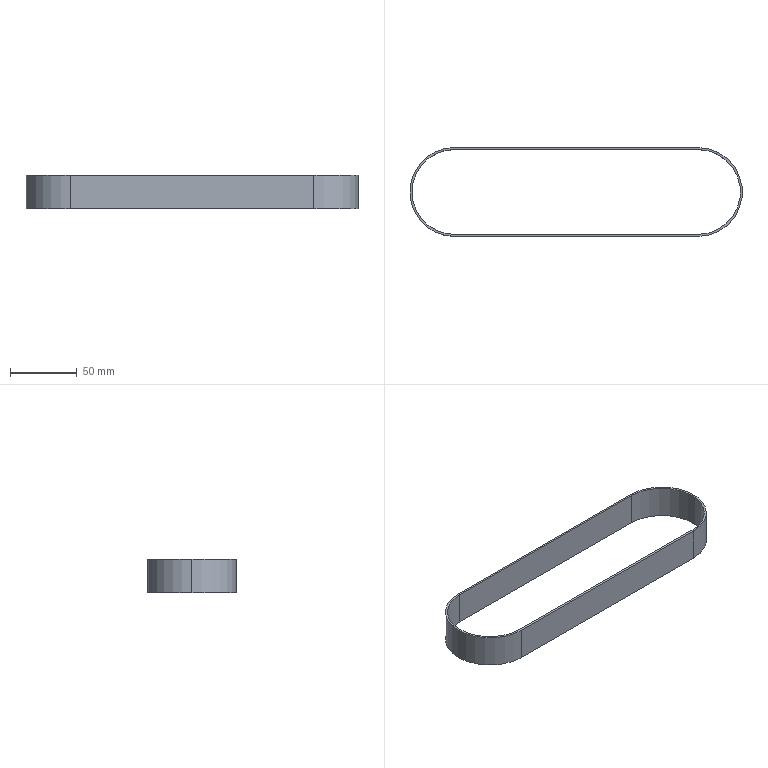Part | STEP file | Timing belt S5M-width 25-length 565 (steel wire core) | 1 solid | 12 faces | box 249.2 x 66.7 x 25 mm | volume 21369 mm3 | cylinder 6 | plane 6 | commonest cylinder face diameters 63.7 x3 66.7 x3
STEP:
#1=CARTESIAN_POINT('',(0.,0.,0.));
#2=DIRECTION('',(0.,0.,1.));
#3=DIRECTION('',(1.,0.,0.));
#4=AXIS2_PLACEMENT_3D('',#1,#2,#3);
#5=CARTESIAN_POINT('',(-91.25,31.85,12.5));
#6=VERTEX_POINT('',#5);
#7=CARTESIAN_POINT('',(-91.25,31.85,-12.5));
#8=VERTEX_POINT('',#7);
#9=CARTESIAN_POINT('',(-91.25,31.85,12.5));
#10=DIRECTION('',(0.,0.,-1.));
#11=VECTOR('',#10,1.);
#12=LINE('',#9,#11);
#13=CARTESIAN_POINT('',(-91.25,0.,12.5));
#14=DIRECTION('',(0.,0.,-1.));
#15=DIRECTION('',(-1.,0.,0.));
#16=AXIS2_PLACEMENT_3D('',#13,#14,#15);
#17=CYLINDRICAL_SURFACE('',#16,31.85);
#18=CARTESIAN_POINT('',(1.571,0.));
#19=DIRECTION('',(0.,1.));
#20=VECTOR('',#19,1.);
#21=LINE('',#18,#20);
#22=(GEOMETRIC_REPRESENTATION_CONTEXT(2)PARAMETRIC_REPRESENTATION_CONTEXT()REPRESENTATION_CONTEXT('',''));
#23=DEFINITIONAL_REPRESENTATION('',(#21),#22);
#24=PCURVE('',#17,#23);
#25=CARTESIAN_POINT('',(-91.25,31.85,12.5));
#26=DIRECTION('',(0.,-1.,0.));
#27=DIRECTION('',(0.,0.,-1.));
#28=AXIS2_PLACEMENT_3D('',#25,#26,#27);
#29=PLANE('',#28);
#30=CARTESIAN_POINT('',(0.,0.));
#31=DIRECTION('',(1.,0.));
#32=VECTOR('',#31,1.);
#33=LINE('',#30,#32);
#34=(GEOMETRIC_REPRESENTATION_CONTEXT(2)PARAMETRIC_REPRESENTATION_CONTEXT()REPRESENTATION_CONTEXT('',''));
#35=DEFINITIONAL_REPRESENTATION('',(#33),#34);
#36=PCURVE('',#29,#35);
#37=SURFACE_CURVE('',#12,(#24,#36),.PCURVE_S1.);
#38=EDGE_CURVE('',#6,#8,#37,.T.);
#39=ORIENTED_EDGE('',*,*,#38,.T.);
#40=CARTESIAN_POINT('',(-123.1,0.,-12.5));
#41=VERTEX_POINT('',#40);
#42=CARTESIAN_POINT('',(-91.25,0.,-12.5));
#43=DIRECTION('',(0.,0.,1.));
#44=DIRECTION('',(1.,0.,0.));
#45=AXIS2_PLACEMENT_3D('',#42,#43,#44);
#46=CIRCLE('',#45,31.85);
#47=CARTESIAN_POINT('',(3.142,25.));
#48=DIRECTION('',(-1.,0.));
#49=VECTOR('',#48,1.);
#50=LINE('',#47,#49);
#51=(GEOMETRIC_REPRESENTATION_CONTEXT(2)PARAMETRIC_REPRESENTATION_CONTEXT()REPRESENTATION_CONTEXT('',''));
#52=DEFINITIONAL_REPRESENTATION('',(#50),#51);
#53=PCURVE('',#17,#52);
#54=CARTESIAN_POINT('',(-91.25,0.,-12.5));
#55=DIRECTION('',(0.,0.,1.));
#56=DIRECTION('',(1.,0.,0.));
#57=AXIS2_PLACEMENT_3D('',#54,#55,#56);
#58=PLANE('',#57);
#59=CARTESIAN_POINT('',(0.,0.));
#60=DIRECTION('',(1.,0.));
#61=AXIS2_PLACEMENT_2D('',#59,#60);
#62=CIRCLE('',#61,31.85);
#63=(GEOMETRIC_REPRESENTATION_CONTEXT(2)PARAMETRIC_REPRESENTATION_CONTEXT()REPRESENTATION_CONTEXT('',''));
#64=DEFINITIONAL_REPRESENTATION('',(#62),#63);
#65=PCURVE('',#58,#64);
#66=SURFACE_CURVE('',#46,(#53,#65),.PCURVE_S1.);
#67=EDGE_CURVE('',#8,#41,#66,.T.);
#68=ORIENTED_EDGE('',*,*,#67,.T.);
#69=CARTESIAN_POINT('',(-123.1,0.,12.5));
#70=VERTEX_POINT('',#69);
#71=CARTESIAN_POINT('',(-123.1,0.,12.5));
#72=DIRECTION('',(0.,0.,-1.));
#73=VECTOR('',#72,1.);
#74=LINE('',#71,#73);
#75=CARTESIAN_POINT('',(0.,0.));
#76=DIRECTION('',(0.,1.));
#77=VECTOR('',#76,1.);
#78=LINE('',#75,#77);
#79=(GEOMETRIC_REPRESENTATION_CONTEXT(2)PARAMETRIC_REPRESENTATION_CONTEXT()REPRESENTATION_CONTEXT('',''));
#80=DEFINITIONAL_REPRESENTATION('',(#78),#79);
#81=PCURVE('',#17,#80);
#82=CARTESIAN_POINT('',(-91.25,0.,12.5));
#83=DIRECTION('',(0.,0.,-1.));
#84=DIRECTION('',(-1.,0.,0.));
#85=AXIS2_PLACEMENT_3D('',#82,#83,#84);
#86=CYLINDRICAL_SURFACE('',#85,31.85);
#87=CARTESIAN_POINT('',(6.283,0.));
#88=DIRECTION('',(0.,1.));
#89=VECTOR('',#88,1.);
#90=LINE('',#87,#89);
#91=(GEOMETRIC_REPRESENTATION_CONTEXT(2)PARAMETRIC_REPRESENTATION_CONTEXT()REPRESENTATION_CONTEXT('',''));
#92=DEFINITIONAL_REPRESENTATION('',(#90),#91);
#93=PCURVE('',#86,#92);
#94=SURFACE_CURVE('',#74,(#81,#93),.PCURVE_S1.);
#95=EDGE_CURVE('',#70,#41,#94,.T.);
#96=ORIENTED_EDGE('',*,*,#95,.F.);
#97=CARTESIAN_POINT('',(-91.25,0.,12.5));
#98=DIRECTION('',(0.,0.,1.));
#99=DIRECTION('',(1.,0.,0.));
#100=AXIS2_PLACEMENT_3D('',#97,#98,#99);
#101=CIRCLE('',#100,31.85);
#102=CARTESIAN_POINT('',(3.142,0.));
#103=DIRECTION('',(-1.,0.));
#104=VECTOR('',#103,1.);
#105=LINE('',#102,#104);
#106=(GEOMETRIC_REPRESENTATION_CONTEXT(2)PARAMETRIC_REPRESENTATION_CONTEXT()REPRESENTATION_CONTEXT('',''));
#107=DEFINITIONAL_REPRESENTATION('',(#105),#106);
#108=PCURVE('',#17,#107);
#109=CARTESIAN_POINT('',(-91.25,0.,12.5));
#110=DIRECTION('',(0.,0.,1.));
#111=DIRECTION('',(1.,0.,0.));
#112=AXIS2_PLACEMENT_3D('',#109,#110,#111);
#113=PLANE('',#112);
#114=CARTESIAN_POINT('',(0.,0.));
#115=DIRECTION('',(1.,0.));
#116=AXIS2_PLACEMENT_2D('',#114,#115);
#117=CIRCLE('',#116,31.85);
#118=(GEOMETRIC_REPRESENTATION_CONTEXT(2)PARAMETRIC_REPRESENTATION_CONTEXT()REPRESENTATION_CONTEXT('',''));
#119=DEFINITIONAL_REPRESENTATION('',(#117),#118);
#120=PCURVE('',#113,#119);
#121=SURFACE_CURVE('',#101,(#108,#120),.PCURVE_S1.);
#122=EDGE_CURVE('',#6,#70,#121,.T.);
#123=ORIENTED_EDGE('',*,*,#122,.F.);
#124=EDGE_LOOP('',(#39,#68,#96,#123));
#125=FACE_BOUND('',#124,.F.);
#126=ADVANCED_FACE('',(#125),#17,.F.);
#127=CARTESIAN_POINT('',(-124.6,0.,12.5));
#128=VERTEX_POINT('',#127);
#129=CARTESIAN_POINT('',(-91.25,-33.35,12.5));
#130=VERTEX_POINT('',#129);
#131=CARTESIAN_POINT('',(-91.25,0.,12.5));
#132=DIRECTION('',(0.,0.,1.));
#133=DIRECTION('',(1.,0.,0.));
#134=AXIS2_PLACEMENT_3D('',#131,#132,#133);
#135=CIRCLE('',#134,33.35);
#136=CARTESIAN_POINT('',(-91.25,0.,12.5));
#137=DIRECTION('',(0.,0.,-1.));
#138=DIRECTION('',(-1.,0.,0.));
#139=AXIS2_PLACEMENT_3D('',#136,#137,#138);
#140=CYLINDRICAL_SURFACE('',#139,33.35);
#141=CARTESIAN_POINT('',(9.425,0.));
#142=DIRECTION('',(-1.,0.));
#143=VECTOR('',#142,1.);
#144=LINE('',#141,#143);
#145=(GEOMETRIC_REPRESENTATION_CONTEXT(2)PARAMETRIC_REPRESENTATION_CONTEXT()REPRESENTATION_CONTEXT('',''));
#146=DEFINITIONAL_REPRESENTATION('',(#144),#145);
#147=PCURVE('',#140,#146);
#148=CARTESIAN_POINT('',(0.,0.));
#149=DIRECTION('',(1.,0.));
#150=AXIS2_PLACEMENT_2D('',#148,#149);
#151=CIRCLE('',#150,33.35);
#152=(GEOMETRIC_REPRESENTATION_CONTEXT(2)PARAMETRIC_REPRESENTATION_CONTEXT()REPRESENTATION_CONTEXT('',''));
#153=DEFINITIONAL_REPRESENTATION('',(#151),#152);
#154=PCURVE('',#113,#153);
#155=SURFACE_CURVE('',#135,(#147,#154),.PCURVE_S1.);
#156=EDGE_CURVE('',#128,#130,#155,.T.);
#157=ORIENTED_EDGE('',*,*,#156,.F.);
#158=CARTESIAN_POINT('',(-124.6,0.,-12.5));
#159=VERTEX_POINT('',#158);
#160=CARTESIAN_POINT('',(-124.6,0.,12.5));
#161=DIRECTION('',(0.,0.,-1.));
#162=VECTOR('',#161,1.);
#163=LINE('',#160,#162);
#164=CARTESIAN_POINT('',(6.283,0.));
#165=DIRECTION('',(0.,1.));
#166=VECTOR('',#165,1.);
#167=LINE('',#164,#166);
#168=(GEOMETRIC_REPRESENTATION_CONTEXT(2)PARAMETRIC_REPRESENTATION_CONTEXT()REPRESENTATION_CONTEXT('',''));
#169=DEFINITIONAL_REPRESENTATION('',(#167),#168);
#170=PCURVE('',#140,#169);
#171=CARTESIAN_POINT('',(-91.25,0.,12.5));
#172=DIRECTION('',(0.,0.,-1.));
#173=DIRECTION('',(-1.,0.,0.));
#174=AXIS2_PLACEMENT_3D('',#171,#172,#173);
#175=CYLINDRICAL_SURFACE('',#174,33.35);
#176=CARTESIAN_POINT('',(0.,0.));
#177=DIRECTION('',(0.,1.));
#178=VECTOR('',#177,1.);
#179=LINE('',#176,#178);
#180=(GEOMETRIC_REPRESENTATION_CONTEXT(2)PARAMETRIC_REPRESENTATION_CONTEXT()REPRESENTATION_CONTEXT('',''));
#181=DEFINITIONAL_REPRESENTATION('',(#179),#180);
#182=PCURVE('',#175,#181);
#183=SURFACE_CURVE('',#163,(#170,#182),.PCURVE_S1.);
#184=EDGE_CURVE('',#128,#159,#183,.T.);
#185=ORIENTED_EDGE('',*,*,#184,.T.);
#186=CARTESIAN_POINT('',(-91.25,-33.35,-12.5));
#187=VERTEX_POINT('',#186);
#188=CARTESIAN_POINT('',(-91.25,0.,-12.5));
#189=DIRECTION('',(0.,0.,1.));
#190=DIRECTION('',(1.,0.,0.));
#191=AXIS2_PLACEMENT_3D('',#188,#189,#190);
#192=CIRCLE('',#191,33.35);
#193=CARTESIAN_POINT('',(9.425,25.));
#194=DIRECTION('',(-1.,0.));
#195=VECTOR('',#194,1.);
#196=LINE('',#193,#195);
#197=(GEOMETRIC_REPRESENTATION_CONTEXT(2)PARAMETRIC_REPRESENTATION_CONTEXT()REPRESENTATION_CONTEXT('',''));
#198=DEFINITIONAL_REPRESENTATION('',(#196),#197);
#199=PCURVE('',#140,#198);
#200=CARTESIAN_POINT('',(0.,0.));
#201=DIRECTION('',(1.,0.));
#202=AXIS2_PLACEMENT_2D('',#200,#201);
#203=CIRCLE('',#202,33.35);
#204=(GEOMETRIC_REPRESENTATION_CONTEXT(2)PARAMETRIC_REPRESENTATION_CONTEXT()REPRESENTATION_CONTEXT('',''));
#205=DEFINITIONAL_REPRESENTATION('',(#203),#204);
#206=PCURVE('',#58,#205);
#207=SURFACE_CURVE('',#192,(#199,#206),.PCURVE_S1.);
#208=EDGE_CURVE('',#159,#187,#207,.T.);
#209=ORIENTED_EDGE('',*,*,#208,.T.);
#210=CARTESIAN_POINT('',(-91.25,-33.35,12.5));
#211=DIRECTION('',(0.,0.,-1.));
#212=VECTOR('',#211,1.);
#213=LINE('',#210,#212);
#214=CARTESIAN_POINT('',(4.712,0.));
#215=DIRECTION('',(0.,1.));
#216=VECTOR('',#215,1.);
#217=LINE('',#214,#216);
#218=(GEOMETRIC_REPRESENTATION_CONTEXT(2)PARAMETRIC_REPRESENTATION_CONTEXT()REPRESENTATION_CONTEXT('',''));
#219=DEFINITIONAL_REPRESENTATION('',(#217),#218);
#220=PCURVE('',#140,#219);
#221=CARTESIAN_POINT('',(-91.25,-33.35,12.5));
#222=DIRECTION('',(0.,1.,0.));
#223=DIRECTION('',(0.,0.,1.));
#224=AXIS2_PLACEMENT_3D('',#221,#222,#223);
#225=PLANE('',#224);
#226=CARTESIAN_POINT('',(0.,0.));
#227=DIRECTION('',(-1.,0.));
#228=VECTOR('',#227,1.);
#229=LINE('',#226,#228);
#230=(GEOMETRIC_REPRESENTATION_CONTEXT(2)PARAMETRIC_REPRESENTATION_CONTEXT()REPRESENTATION_CONTEXT('',''));
#231=DEFINITIONAL_REPRESENTATION('',(#229),#230);
#232=PCURVE('',#225,#231);
#233=SURFACE_CURVE('',#213,(#220,#232),.PCURVE_S1.);
#234=EDGE_CURVE('',#130,#187,#233,.T.);
#235=ORIENTED_EDGE('',*,*,#234,.F.);
#236=EDGE_LOOP('',(#157,#185,#209,#235));
#237=FACE_BOUND('',#236,.T.);
#238=ADVANCED_FACE('',(#237),#140,.T.);
#239=CARTESIAN_POINT('',(-91.25,33.35,12.5));
#240=VERTEX_POINT('',#239);
#241=CARTESIAN_POINT('',(-91.25,0.,12.5));
#242=DIRECTION('',(0.,0.,1.));
#243=DIRECTION('',(1.,0.,0.));
#244=AXIS2_PLACEMENT_3D('',#241,#242,#243);
#245=CIRCLE('',#244,33.35);
#246=CARTESIAN_POINT('',(0.,0.));
#247=DIRECTION('',(1.,0.));
#248=AXIS2_PLACEMENT_2D('',#246,#247);
#249=CIRCLE('',#248,33.35);
#250=(GEOMETRIC_REPRESENTATION_CONTEXT(2)PARAMETRIC_REPRESENTATION_CONTEXT()REPRESENTATION_CONTEXT('',''));
#251=DEFINITIONAL_REPRESENTATION('',(#249),#250);
#252=PCURVE('',#113,#251);
#253=CARTESIAN_POINT('',(3.142,0.));
#254=DIRECTION('',(-1.,0.));
#255=VECTOR('',#254,1.);
#256=LINE('',#253,#255);
#257=(GEOMETRIC_REPRESENTATION_CONTEXT(2)PARAMETRIC_REPRESENTATION_CONTEXT()REPRESENTATION_CONTEXT('',''));
#258=DEFINITIONAL_REPRESENTATION('',(#256),#257);
#259=PCURVE('',#175,#258);
#260=SURFACE_CURVE('',#245,(#252,#259),.PCURVE_S1.);
#261=EDGE_CURVE('',#240,#128,#260,.T.);
#262=ORIENTED_EDGE('',*,*,#261,.T.);
#263=ORIENTED_EDGE('',*,*,#156,.T.);
#264=CARTESIAN_POINT('',(91.25,-33.35,12.5));
#265=VERTEX_POINT('',#264);
#266=CARTESIAN_POINT('',(-91.25,-33.35,12.5));
#267=DIRECTION('',(1.,0.,0.));
#268=VECTOR('',#267,1.);
#269=LINE('',#266,#268);
#270=CARTESIAN_POINT('',(0.,-33.35));
#271=DIRECTION('',(1.,0.));
#272=VECTOR('',#271,1.);
#273=LINE('',#270,#272);
#274=(GEOMETRIC_REPRESENTATION_CONTEXT(2)PARAMETRIC_REPRESENTATION_CONTEXT()REPRESENTATION_CONTEXT('',''));
#275=DEFINITIONAL_REPRESENTATION('',(#273),#274);
#276=PCURVE('',#113,#275);
#277=CARTESIAN_POINT('',(0.,0.));
#278=DIRECTION('',(0.,1.));
#279=VECTOR('',#278,1.);
#280=LINE('',#277,#279);
#281=(GEOMETRIC_REPRESENTATION_CONTEXT(2)PARAMETRIC_REPRESENTATION_CONTEXT()REPRESENTATION_CONTEXT('',''));
#282=DEFINITIONAL_REPRESENTATION('',(#280),#281);
#283=PCURVE('',#225,#282);
#284=SURFACE_CURVE('',#269,(#276,#283),.PCURVE_S1.);
#285=EDGE_CURVE('',#130,#265,#284,.T.);
#286=ORIENTED_EDGE('',*,*,#285,.T.);
#287=CARTESIAN_POINT('',(91.25,33.35,12.5));
#288=VERTEX_POINT('',#287);
#289=CARTESIAN_POINT('',(91.25,0.,12.5));
#290=DIRECTION('',(0.,0.,1.));
#291=DIRECTION('',(1.,0.,0.));
#292=AXIS2_PLACEMENT_3D('',#289,#290,#291);
#293=CIRCLE('',#292,33.35);
#294=CARTESIAN_POINT('',(182.5,0.));
#295=DIRECTION('',(1.,0.));
#296=AXIS2_PLACEMENT_2D('',#294,#295);
#297=CIRCLE('',#296,33.35);
#298=(GEOMETRIC_REPRESENTATION_CONTEXT(2)PARAMETRIC_REPRESENTATION_CONTEXT()REPRESENTATION_CONTEXT('',''));
#299=DEFINITIONAL_REPRESENTATION('',(#297),#298);
#300=PCURVE('',#113,#299);
#301=CARTESIAN_POINT('',(91.25,0.,12.5));
#302=DIRECTION('',(0.,0.,-1.));
#303=DIRECTION('',(-1.,0.,0.));
#304=AXIS2_PLACEMENT_3D('',#301,#302,#303);
#305=CYLINDRICAL_SURFACE('',#304,33.35);
#306=CARTESIAN_POINT('',(9.425,0.));
#307=DIRECTION('',(-1.,0.));
#308=VECTOR('',#307,1.);
#309=LINE('',#306,#308);
#310=(GEOMETRIC_REPRESENTATION_CONTEXT(2)PARAMETRIC_REPRESENTATION_CONTEXT()REPRESENTATION_CONTEXT('',''));
#311=DEFINITIONAL_REPRESENTATION('',(#309),#310);
#312=PCURVE('',#305,#311);
#313=SURFACE_CURVE('',#293,(#300,#312),.PCURVE_S1.);
#314=EDGE_CURVE('',#265,#288,#313,.T.);
#315=ORIENTED_EDGE('',*,*,#314,.T.);
#316=CARTESIAN_POINT('',(-91.25,33.35,12.5));
#317=DIRECTION('',(-1.,0.,0.));
#318=VECTOR('',#317,1.);
#319=LINE('',#316,#318);
#320=CARTESIAN_POINT('',(0.,33.35));
#321=DIRECTION('',(-1.,0.));
#322=VECTOR('',#321,1.);
#323=LINE('',#320,#322);
#324=(GEOMETRIC_REPRESENTATION_CONTEXT(2)PARAMETRIC_REPRESENTATION_CONTEXT()REPRESENTATION_CONTEXT('',''));
#325=DEFINITIONAL_REPRESENTATION('',(#323),#324);
#326=PCURVE('',#113,#325);
#327=CARTESIAN_POINT('',(-91.25,33.35,12.5));
#328=DIRECTION('',(0.,-1.,0.));
#329=DIRECTION('',(0.,0.,-1.));
#330=AXIS2_PLACEMENT_3D('',#327,#328,#329);
#331=PLANE('',#330);
#332=CARTESIAN_POINT('',(0.,0.));
#333=DIRECTION('',(0.,-1.));
#334=VECTOR('',#333,1.);
#335=LINE('',#332,#334);
#336=(GEOMETRIC_REPRESENTATION_CONTEXT(2)PARAMETRIC_REPRESENTATION_CONTEXT()REPRESENTATION_CONTEXT('',''));
#337=DEFINITIONAL_REPRESENTATION('',(#335),#336);
#338=PCURVE('',#331,#337);
#339=SURFACE_CURVE('',#319,(#326,#338),.PCURVE_S1.);
#340=EDGE_CURVE('',#288,#240,#339,.T.);
#341=ORIENTED_EDGE('',*,*,#340,.T.);
#342=EDGE_LOOP('',(#262,#263,#286,#315,#341));
#343=FACE_BOUND('',#342,.T.);
#344=CARTESIAN_POINT('',(-91.25,-31.85,12.5));
#345=VERTEX_POINT('',#344);
#346=CARTESIAN_POINT('',(91.25,-31.85,12.5));
#347=VERTEX_POINT('',#346);
#348=CARTESIAN_POINT('',(-91.25,-31.85,12.5));
#349=DIRECTION('',(1.,0.,0.));
#350=VECTOR('',#349,1.);
#351=LINE('',#348,#350);
#352=CARTESIAN_POINT('',(0.,-31.85));
#353=DIRECTION('',(1.,0.));
#354=VECTOR('',#353,1.);
#355=LINE('',#352,#354);
#356=(GEOMETRIC_REPRESENTATION_CONTEXT(2)PARAMETRIC_REPRESENTATION_CONTEXT()REPRESENTATION_CONTEXT('',''));
#357=DEFINITIONAL_REPRESENTATION('',(#355),#356);
#358=PCURVE('',#113,#357);
#359=CARTESIAN_POINT('',(-91.25,-31.85,12.5));
#360=DIRECTION('',(0.,1.,0.));
#361=DIRECTION('',(0.,0.,1.));
#362=AXIS2_PLACEMENT_3D('',#359,#360,#361);
#363=PLANE('',#362);
#364=CARTESIAN_POINT('',(0.,0.));
#365=DIRECTION('',(0.,1.));
#366=VECTOR('',#365,1.);
#367=LINE('',#364,#366);
#368=(GEOMETRIC_REPRESENTATION_CONTEXT(2)PARAMETRIC_REPRESENTATION_CONTEXT()REPRESENTATION_CONTEXT('',''));
#369=DEFINITIONAL_REPRESENTATION('',(#367),#368);
#370=PCURVE('',#363,#369);
#371=SURFACE_CURVE('',#351,(#358,#370),.PCURVE_S1.);
#372=EDGE_CURVE('',#345,#347,#371,.T.);
#373=ORIENTED_EDGE('',*,*,#372,.F.);
#374=CARTESIAN_POINT('',(-91.25,0.,12.5));
#375=DIRECTION('',(0.,0.,1.));
#376=DIRECTION('',(1.,0.,0.));
#377=AXIS2_PLACEMENT_3D('',#374,#375,#376);
#378=CIRCLE('',#377,31.85);
#379=CARTESIAN_POINT('',(0.,0.));
#380=DIRECTION('',(1.,0.));
#381=AXIS2_PLACEMENT_2D('',#379,#380);
#382=CIRCLE('',#381,31.85);
#383=(GEOMETRIC_REPRESENTATION_CONTEXT(2)PARAMETRIC_REPRESENTATION_CONTEXT()REPRESENTATION_CONTEXT('',''));
#384=DEFINITIONAL_REPRESENTATION('',(#382),#383);
#385=PCURVE('',#113,#384);
#386=CARTESIAN_POINT('',(9.425,0.));
#387=DIRECTION('',(-1.,0.));
#388=VECTOR('',#387,1.);
#389=LINE('',#386,#388);
#390=(GEOMETRIC_REPRESENTATION_CONTEXT(2)PARAMETRIC_REPRESENTATION_CONTEXT()REPRESENTATION_CONTEXT('',''));
#391=DEFINITIONAL_REPRESENTATION('',(#389),#390);
#392=PCURVE('',#86,#391);
#393=SURFACE_CURVE('',#378,(#385,#392),.PCURVE_S1.);
#394=EDGE_CURVE('',#70,#345,#393,.T.);
#395=ORIENTED_EDGE('',*,*,#394,.F.);
#396=ORIENTED_EDGE('',*,*,#122,.F.);
#397=CARTESIAN_POINT('',(91.25,31.85,12.5));
#398=VERTEX_POINT('',#397);
#399=CARTESIAN_POINT('',(-91.25,31.85,12.5));
#400=DIRECTION('',(-1.,0.,0.));
#401=VECTOR('',#400,1.);
#402=LINE('',#399,#401);
#403=CARTESIAN_POINT('',(0.,31.85));
#404=DIRECTION('',(-1.,0.));
#405=VECTOR('',#404,1.);
#406=LINE('',#403,#405);
#407=(GEOMETRIC_REPRESENTATION_CONTEXT(2)PARAMETRIC_REPRESENTATION_CONTEXT()REPRESENTATION_CONTEXT('',''));
#408=DEFINITIONAL_REPRESENTATION('',(#406),#407);
#409=PCURVE('',#113,#408);
#410=CARTESIAN_POINT('',(0.,0.));
#411=DIRECTION('',(0.,-1.));
#412=VECTOR('',#411,1.);
#413=LINE('',#410,#412);
#414=(GEOMETRIC_REPRESENTATION_CONTEXT(2)PARAMETRIC_REPRESENTATION_CONTEXT()REPRESENTATION_CONTEXT('',''));
#415=DEFINITIONAL_REPRESENTATION('',(#413),#414);
#416=PCURVE('',#29,#415);
#417=SURFACE_CURVE('',#402,(#409,#416),.PCURVE_S1.);
#418=EDGE_CURVE('',#398,#6,#417,.T.);
#419=ORIENTED_EDGE('',*,*,#418,.F.);
#420=CARTESIAN_POINT('',(91.25,0.,12.5));
#421=DIRECTION('',(0.,0.,1.));
#422=DIRECTION('',(1.,0.,0.));
#423=AXIS2_PLACEMENT_3D('',#420,#421,#422);
#424=CIRCLE('',#423,31.85);
#425=CARTESIAN_POINT('',(182.5,0.));
#426=DIRECTION('',(1.,0.));
#427=AXIS2_PLACEMENT_2D('',#425,#426);
#428=CIRCLE('',#427,31.85);
#429=(GEOMETRIC_REPRESENTATION_CONTEXT(2)PARAMETRIC_REPRESENTATION_CONTEXT()REPRESENTATION_CONTEXT('',''));
#430=DEFINITIONAL_REPRESENTATION('',(#428),#429);
#431=PCURVE('',#113,#430);
#432=CARTESIAN_POINT('',(91.25,0.,12.5));
#433=DIRECTION('',(0.,0.,-1.));
#434=DIRECTION('',(-1.,0.,0.));
#435=AXIS2_PLACEMENT_3D('',#432,#433,#434);
#436=CYLINDRICAL_SURFACE('',#435,31.85);
#437=CARTESIAN_POINT('',(9.425,0.));
#438=DIRECTION('',(-1.,0.));
#439=VECTOR('',#438,1.);
#440=LINE('',#437,#439);
#441=(GEOMETRIC_REPRESENTATION_CONTEXT(2)PARAMETRIC_REPRESENTATION_CONTEXT()REPRESENTATION_CONTEXT('',''));
#442=DEFINITIONAL_REPRESENTATION('',(#440),#441);
#443=PCURVE('',#436,#442);
#444=SURFACE_CURVE('',#424,(#431,#443),.PCURVE_S1.);
#445=EDGE_CURVE('',#347,#398,#444,.T.);
#446=ORIENTED_EDGE('',*,*,#445,.F.);
#447=EDGE_LOOP('',(#373,#395,#396,#419,#446));
#448=FACE_BOUND('',#447,.T.);
#449=ADVANCED_FACE('',(#343,#448),#113,.T.);
#450=CARTESIAN_POINT('',(-91.25,33.35,-12.5));
#451=VERTEX_POINT('',#450);
#452=CARTESIAN_POINT('',(-91.25,0.,-12.5));
#453=DIRECTION('',(0.,0.,1.));
#454=DIRECTION('',(1.,0.,0.));
#455=AXIS2_PLACEMENT_3D('',#452,#453,#454);
#456=CIRCLE('',#455,33.35);
#457=CARTESIAN_POINT('',(0.,0.));
#458=DIRECTION('',(1.,0.));
#459=AXIS2_PLACEMENT_2D('',#457,#458);
#460=CIRCLE('',#459,33.35);
#461=(GEOMETRIC_REPRESENTATION_CONTEXT(2)PARAMETRIC_REPRESENTATION_CONTEXT()REPRESENTATION_CONTEXT('',''));
#462=DEFINITIONAL_REPRESENTATION('',(#460),#461);
#463=PCURVE('',#58,#462);
#464=CARTESIAN_POINT('',(3.142,25.));
#465=DIRECTION('',(-1.,0.));
#466=VECTOR('',#465,1.);
#467=LINE('',#464,#466);
#468=(GEOMETRIC_REPRESENTATION_CONTEXT(2)PARAMETRIC_REPRESENTATION_CONTEXT()REPRESENTATION_CONTEXT('',''));
#469=DEFINITIONAL_REPRESENTATION('',(#467),#468);
#470=PCURVE('',#175,#469);
#471=SURFACE_CURVE('',#456,(#463,#470),.PCURVE_S1.);
#472=EDGE_CURVE('',#451,#159,#471,.T.);
#473=ORIENTED_EDGE('',*,*,#472,.F.);
#474=CARTESIAN_POINT('',(91.25,33.35,-12.5));
#475=VERTEX_POINT('',#474);
#476=CARTESIAN_POINT('',(-91.25,33.35,-12.5));
#477=DIRECTION('',(-1.,0.,0.));
#478=VECTOR('',#477,1.);
#479=LINE('',#476,#478);
#480=CARTESIAN_POINT('',(0.,33.35));
#481=DIRECTION('',(-1.,0.));
#482=VECTOR('',#481,1.);
#483=LINE('',#480,#482);
#484=(GEOMETRIC_REPRESENTATION_CONTEXT(2)PARAMETRIC_REPRESENTATION_CONTEXT()REPRESENTATION_CONTEXT('',''));
#485=DEFINITIONAL_REPRESENTATION('',(#483),#484);
#486=PCURVE('',#58,#485);
#487=CARTESIAN_POINT('',(25.,0.));
#488=DIRECTION('',(0.,-1.));
#489=VECTOR('',#488,1.);
#490=LINE('',#487,#489);
#491=(GEOMETRIC_REPRESENTATION_CONTEXT(2)PARAMETRIC_REPRESENTATION_CONTEXT()REPRESENTATION_CONTEXT('',''));
#492=DEFINITIONAL_REPRESENTATION('',(#490),#491);
#493=PCURVE('',#331,#492);
#494=SURFACE_CURVE('',#479,(#486,#493),.PCURVE_S1.);
#495=EDGE_CURVE('',#475,#451,#494,.T.);
#496=ORIENTED_EDGE('',*,*,#495,.F.);
#497=CARTESIAN_POINT('',(91.25,-33.35,-12.5));
#498=VERTEX_POINT('',#497);
#499=CARTESIAN_POINT('',(91.25,0.,-12.5));
#500=DIRECTION('',(0.,0.,1.));
#501=DIRECTION('',(1.,0.,0.));
#502=AXIS2_PLACEMENT_3D('',#499,#500,#501);
#503=CIRCLE('',#502,33.35);
#504=CARTESIAN_POINT('',(182.5,0.));
#505=DIRECTION('',(1.,0.));
#506=AXIS2_PLACEMENT_2D('',#504,#505);
#507=CIRCLE('',#506,33.35);
#508=(GEOMETRIC_REPRESENTATION_CONTEXT(2)PARAMETRIC_REPRESENTATION_CONTEXT()REPRESENTATION_CONTEXT('',''));
#509=DEFINITIONAL_REPRESENTATION('',(#507),#508);
#510=PCURVE('',#58,#509);
#511=CARTESIAN_POINT('',(9.425,25.));
#512=DIRECTION('',(-1.,0.));
#513=VECTOR('',#512,1.);
#514=LINE('',#511,#513);
#515=(GEOMETRIC_REPRESENTATION_CONTEXT(2)PARAMETRIC_REPRESENTATION_CONTEXT()REPRESENTATION_CONTEXT('',''));
#516=DEFINITIONAL_REPRESENTATION('',(#514),#515);
#517=PCURVE('',#305,#516);
#518=SURFACE_CURVE('',#503,(#510,#517),.PCURVE_S1.);
#519=EDGE_CURVE('',#498,#475,#518,.T.);
#520=ORIENTED_EDGE('',*,*,#519,.F.);
#521=CARTESIAN_POINT('',(-91.25,-33.35,-12.5));
#522=DIRECTION('',(1.,0.,0.));
#523=VECTOR('',#522,1.);
#524=LINE('',#521,#523);
#525=CARTESIAN_POINT('',(0.,-33.35));
#526=DIRECTION('',(1.,0.));
#527=VECTOR('',#526,1.);
#528=LINE('',#525,#527);
#529=(GEOMETRIC_REPRESENTATION_CONTEXT(2)PARAMETRIC_REPRESENTATION_CONTEXT()REPRESENTATION_CONTEXT('',''));
#530=DEFINITIONAL_REPRESENTATION('',(#528),#529);
#531=PCURVE('',#58,#530);
#532=CARTESIAN_POINT('',(-25.,0.));
#533=DIRECTION('',(0.,1.));
#534=VECTOR('',#533,1.);
#535=LINE('',#532,#534);
#536=(GEOMETRIC_REPRESENTATION_CONTEXT(2)PARAMETRIC_REPRESENTATION_CONTEXT()REPRESENTATION_CONTEXT('',''));
#537=DEFINITIONAL_REPRESENTATION('',(#535),#536);
#538=PCURVE('',#225,#537);
#539=SURFACE_CURVE('',#524,(#531,#538),.PCURVE_S1.);
#540=EDGE_CURVE('',#187,#498,#539,.T.);
#541=ORIENTED_EDGE('',*,*,#540,.F.);
#542=ORIENTED_EDGE('',*,*,#208,.F.);
#543=EDGE_LOOP('',(#473,#496,#520,#541,#542));
#544=FACE_BOUND('',#543,.T.);
#545=ORIENTED_EDGE('',*,*,#67,.T.);
#546=CARTESIAN_POINT('',(-91.25,-31.85,-12.5));
#547=VERTEX_POINT('',#546);
#548=CARTESIAN_POINT('',(-91.25,0.,-12.5));
#549=DIRECTION('',(0.,0.,1.));
#550=DIRECTION('',(1.,0.,0.));
#551=AXIS2_PLACEMENT_3D('',#548,#549,#550);
#552=CIRCLE('',#551,31.85);
#553=CARTESIAN_POINT('',(0.,0.));
#554=DIRECTION('',(1.,0.));
#555=AXIS2_PLACEMENT_2D('',#553,#554);
#556=CIRCLE('',#555,31.85);
#557=(GEOMETRIC_REPRESENTATION_CONTEXT(2)PARAMETRIC_REPRESENTATION_CONTEXT()REPRESENTATION_CONTEXT('',''));
#558=DEFINITIONAL_REPRESENTATION('',(#556),#557);
#559=PCURVE('',#58,#558);
#560=CARTESIAN_POINT('',(9.425,25.));
#561=DIRECTION('',(-1.,0.));
#562=VECTOR('',#561,1.);
#563=LINE('',#560,#562);
#564=(GEOMETRIC_REPRESENTATION_CONTEXT(2)PARAMETRIC_REPRESENTATION_CONTEXT()REPRESENTATION_CONTEXT('',''));
#565=DEFINITIONAL_REPRESENTATION('',(#563),#564);
#566=PCURVE('',#86,#565);
#567=SURFACE_CURVE('',#552,(#559,#566),.PCURVE_S1.);
#568=EDGE_CURVE('',#41,#547,#567,.T.);
#569=ORIENTED_EDGE('',*,*,#568,.T.);
#570=CARTESIAN_POINT('',(91.25,-31.85,-12.5));
#571=VERTEX_POINT('',#570);
#572=CARTESIAN_POINT('',(-91.25,-31.85,-12.5));
#573=DIRECTION('',(1.,0.,0.));
#574=VECTOR('',#573,1.);
#575=LINE('',#572,#574);
#576=CARTESIAN_POINT('',(0.,-31.85));
#577=DIRECTION('',(1.,0.));
#578=VECTOR('',#577,1.);
#579=LINE('',#576,#578);
#580=(GEOMETRIC_REPRESENTATION_CONTEXT(2)PARAMETRIC_REPRESENTATION_CONTEXT()REPRESENTATION_CONTEXT('',''));
#581=DEFINITIONAL_REPRESENTATION('',(#579),#580);
#582=PCURVE('',#58,#581);
#583=CARTESIAN_POINT('',(-25.,0.));
#584=DIRECTION('',(0.,1.));
#585=VECTOR('',#584,1.);
#586=LINE('',#583,#585);
#587=(GEOMETRIC_REPRESENTATION_CONTEXT(2)PARAMETRIC_REPRESENTATION_CONTEXT()REPRESENTATION_CONTEXT('',''));
#588=DEFINITIONAL_REPRESENTATION('',(#586),#587);
#589=PCURVE('',#363,#588);
#590=SURFACE_CURVE('',#575,(#582,#589),.PCURVE_S1.);
#591=EDGE_CURVE('',#547,#571,#590,.T.);
#592=ORIENTED_EDGE('',*,*,#591,.T.);
#593=CARTESIAN_POINT('',(91.25,31.85,-12.5));
#594=VERTEX_POINT('',#593);
#595=CARTESIAN_POINT('',(91.25,0.,-12.5));
#596=DIRECTION('',(0.,0.,1.));
#597=DIRECTION('',(1.,0.,0.));
#598=AXIS2_PLACEMENT_3D('',#595,#596,#597);
#599=CIRCLE('',#598,31.85);
#600=CARTESIAN_POINT('',(182.5,0.));
#601=DIRECTION('',(1.,0.));
#602=AXIS2_PLACEMENT_2D('',#600,#601);
#603=CIRCLE('',#602,31.85);
#604=(GEOMETRIC_REPRESENTATION_CONTEXT(2)PARAMETRIC_REPRESENTATION_CONTEXT()REPRESENTATION_CONTEXT('',''));
#605=DEFINITIONAL_REPRESENTATION('',(#603),#604);
#606=PCURVE('',#58,#605);
#607=CARTESIAN_POINT('',(9.425,25.));
#608=DIRECTION('',(-1.,0.));
#609=VECTOR('',#608,1.);
#610=LINE('',#607,#609);
#611=(GEOMETRIC_REPRESENTATION_CONTEXT(2)PARAMETRIC_REPRESENTATION_CONTEXT()REPRESENTATION_CONTEXT('',''));
#612=DEFINITIONAL_REPRESENTATION('',(#610),#611);
#613=PCURVE('',#436,#612);
#614=SURFACE_CURVE('',#599,(#606,#613),.PCURVE_S1.);
#615=EDGE_CURVE('',#571,#594,#614,.T.);
#616=ORIENTED_EDGE('',*,*,#615,.T.);
#617=CARTESIAN_POINT('',(-91.25,31.85,-12.5));
#618=DIRECTION('',(-1.,0.,0.));
#619=VECTOR('',#618,1.);
#620=LINE('',#617,#619);
#621=CARTESIAN_POINT('',(0.,31.85));
#622=DIRECTION('',(-1.,0.));
#623=VECTOR('',#622,1.);
#624=LINE('',#621,#623);
#625=(GEOMETRIC_REPRESENTATION_CONTEXT(2)PARAMETRIC_REPRESENTATION_CONTEXT()REPRESENTATION_CONTEXT('',''));
#626=DEFINITIONAL_REPRESENTATION('',(#624),#625);
#627=PCURVE('',#58,#626);
#628=CARTESIAN_POINT('',(25.,0.));
#629=DIRECTION('',(0.,-1.));
#630=VECTOR('',#629,1.);
#631=LINE('',#628,#630);
#632=(GEOMETRIC_REPRESENTATION_CONTEXT(2)PARAMETRIC_REPRESENTATION_CONTEXT()REPRESENTATION_CONTEXT('',''));
#633=DEFINITIONAL_REPRESENTATION('',(#631),#632);
#634=PCURVE('',#29,#633);
#635=SURFACE_CURVE('',#620,(#627,#634),.PCURVE_S1.);
#636=EDGE_CURVE('',#594,#8,#635,.T.);
#637=ORIENTED_EDGE('',*,*,#636,.T.);
#638=EDGE_LOOP('',(#545,#569,#592,#616,#637));
#639=FACE_BOUND('',#638,.T.);
#640=ADVANCED_FACE('',(#544,#639),#58,.F.);
#641=ORIENTED_EDGE('',*,*,#184,.F.);
#642=ORIENTED_EDGE('',*,*,#261,.F.);
#643=CARTESIAN_POINT('',(-91.25,33.35,12.5));
#644=DIRECTION('',(0.,0.,-1.));
#645=VECTOR('',#644,1.);
#646=LINE('',#643,#645);
#647=CARTESIAN_POINT('',(1.571,0.));
#648=DIRECTION('',(0.,1.));
#649=VECTOR('',#648,1.);
#650=LINE('',#647,#649);
#651=(GEOMETRIC_REPRESENTATION_CONTEXT(2)PARAMETRIC_REPRESENTATION_CONTEXT()REPRESENTATION_CONTEXT('',''));
#652=DEFINITIONAL_REPRESENTATION('',(#650),#651);
#653=PCURVE('',#175,#652);
#654=CARTESIAN_POINT('',(0.,0.));
#655=DIRECTION('',(1.,0.));
#656=VECTOR('',#655,1.);
#657=LINE('',#654,#656);
#658=(GEOMETRIC_REPRESENTATION_CONTEXT(2)PARAMETRIC_REPRESENTATION_CONTEXT()REPRESENTATION_CONTEXT('',''));
#659=DEFINITIONAL_REPRESENTATION('',(#657),#658);
#660=PCURVE('',#331,#659);
#661=SURFACE_CURVE('',#646,(#653,#660),.PCURVE_S1.);
#662=EDGE_CURVE('',#240,#451,#661,.T.);
#663=ORIENTED_EDGE('',*,*,#662,.T.);
#664=ORIENTED_EDGE('',*,*,#472,.T.);
#665=EDGE_LOOP('',(#641,#642,#663,#664));
#666=FACE_BOUND('',#665,.T.);
#667=ADVANCED_FACE('',(#666),#175,.T.);
#668=ORIENTED_EDGE('',*,*,#540,.T.);
#669=CARTESIAN_POINT('',(91.25,-33.35,12.5));
#670=DIRECTION('',(0.,0.,-1.));
#671=VECTOR('',#670,1.);
#672=LINE('',#669,#671);
#673=CARTESIAN_POINT('',(0.,182.5));
#674=DIRECTION('',(-1.,0.));
#675=VECTOR('',#674,1.);
#676=LINE('',#673,#675);
#677=(GEOMETRIC_REPRESENTATION_CONTEXT(2)PARAMETRIC_REPRESENTATION_CONTEXT()REPRESENTATION_CONTEXT('',''));
#678=DEFINITIONAL_REPRESENTATION('',(#676),#677);
#679=PCURVE('',#225,#678);
#680=CARTESIAN_POINT('',(4.712,0.));
#681=DIRECTION('',(0.,1.));
#682=VECTOR('',#681,1.);
#683=LINE('',#680,#682);
#684=(GEOMETRIC_REPRESENTATION_CONTEXT(2)PARAMETRIC_REPRESENTATION_CONTEXT()REPRESENTATION_CONTEXT('',''));
#685=DEFINITIONAL_REPRESENTATION('',(#683),#684);
#686=PCURVE('',#305,#685);
#687=SURFACE_CURVE('',#672,(#679,#686),.PCURVE_S1.);
#688=EDGE_CURVE('',#265,#498,#687,.T.);
#689=ORIENTED_EDGE('',*,*,#688,.F.);
#690=ORIENTED_EDGE('',*,*,#285,.F.);
#691=ORIENTED_EDGE('',*,*,#234,.T.);
#692=EDGE_LOOP('',(#668,#689,#690,#691));
#693=FACE_BOUND('',#692,.T.);
#694=ADVANCED_FACE('',(#693),#225,.F.);
#695=ORIENTED_EDGE('',*,*,#519,.T.);
#696=CARTESIAN_POINT('',(91.25,33.35,12.5));
#697=DIRECTION('',(0.,0.,-1.));
#698=VECTOR('',#697,1.);
#699=LINE('',#696,#698);
#700=CARTESIAN_POINT('',(1.571,0.));
#701=DIRECTION('',(0.,1.));
#702=VECTOR('',#701,1.);
#703=LINE('',#700,#702);
#704=(GEOMETRIC_REPRESENTATION_CONTEXT(2)PARAMETRIC_REPRESENTATION_CONTEXT()REPRESENTATION_CONTEXT('',''));
#705=DEFINITIONAL_REPRESENTATION('',(#703),#704);
#706=PCURVE('',#305,#705);
#707=CARTESIAN_POINT('',(0.,182.5));
#708=DIRECTION('',(1.,0.));
#709=VECTOR('',#708,1.);
#710=LINE('',#707,#709);
#711=(GEOMETRIC_REPRESENTATION_CONTEXT(2)PARAMETRIC_REPRESENTATION_CONTEXT()REPRESENTATION_CONTEXT('',''));
#712=DEFINITIONAL_REPRESENTATION('',(#710),#711);
#713=PCURVE('',#331,#712);
#714=SURFACE_CURVE('',#699,(#706,#713),.PCURVE_S1.);
#715=EDGE_CURVE('',#288,#475,#714,.T.);
#716=ORIENTED_EDGE('',*,*,#715,.F.);
#717=ORIENTED_EDGE('',*,*,#314,.F.);
#718=ORIENTED_EDGE('',*,*,#688,.T.);
#719=EDGE_LOOP('',(#695,#716,#717,#718));
#720=FACE_BOUND('',#719,.T.);
#721=ADVANCED_FACE('',(#720),#305,.T.);
#722=ORIENTED_EDGE('',*,*,#495,.T.);
#723=ORIENTED_EDGE('',*,*,#662,.F.);
#724=ORIENTED_EDGE('',*,*,#340,.F.);
#725=ORIENTED_EDGE('',*,*,#715,.T.);
#726=EDGE_LOOP('',(#722,#723,#724,#725));
#727=FACE_BOUND('',#726,.T.);
#728=ADVANCED_FACE('',(#727),#331,.F.);
#729=ORIENTED_EDGE('',*,*,#568,.T.);
#730=CARTESIAN_POINT('',(-91.25,-31.85,12.5));
#731=DIRECTION('',(0.,0.,-1.));
#732=VECTOR('',#731,1.);
#733=LINE('',#730,#732);
#734=CARTESIAN_POINT('',(4.712,0.));
#735=DIRECTION('',(0.,1.));
#736=VECTOR('',#735,1.);
#737=LINE('',#734,#736);
#738=(GEOMETRIC_REPRESENTATION_CONTEXT(2)PARAMETRIC_REPRESENTATION_CONTEXT()REPRESENTATION_CONTEXT('',''));
#739=DEFINITIONAL_REPRESENTATION('',(#737),#738);
#740=PCURVE('',#86,#739);
#741=CARTESIAN_POINT('',(0.,0.));
#742=DIRECTION('',(-1.,0.));
#743=VECTOR('',#742,1.);
#744=LINE('',#741,#743);
#745=(GEOMETRIC_REPRESENTATION_CONTEXT(2)PARAMETRIC_REPRESENTATION_CONTEXT()REPRESENTATION_CONTEXT('',''));
#746=DEFINITIONAL_REPRESENTATION('',(#744),#745);
#747=PCURVE('',#363,#746);
#748=SURFACE_CURVE('',#733,(#740,#747),.PCURVE_S1.);
#749=EDGE_CURVE('',#345,#547,#748,.T.);
#750=ORIENTED_EDGE('',*,*,#749,.F.);
#751=ORIENTED_EDGE('',*,*,#394,.F.);
#752=ORIENTED_EDGE('',*,*,#95,.T.);
#753=EDGE_LOOP('',(#729,#750,#751,#752));
#754=FACE_BOUND('',#753,.F.);
#755=ADVANCED_FACE('',(#754),#86,.F.);
#756=ORIENTED_EDGE('',*,*,#591,.F.);
#757=ORIENTED_EDGE('',*,*,#749,.F.);
#758=ORIENTED_EDGE('',*,*,#372,.T.);
#759=CARTESIAN_POINT('',(91.25,-31.85,12.5));
#760=DIRECTION('',(0.,0.,-1.));
#761=VECTOR('',#760,1.);
#762=LINE('',#759,#761);
#763=CARTESIAN_POINT('',(0.,182.5));
#764=DIRECTION('',(-1.,0.));
#765=VECTOR('',#764,1.);
#766=LINE('',#763,#765);
#767=(GEOMETRIC_REPRESENTATION_CONTEXT(2)PARAMETRIC_REPRESENTATION_CONTEXT()REPRESENTATION_CONTEXT('',''));
#768=DEFINITIONAL_REPRESENTATION('',(#766),#767);
#769=PCURVE('',#363,#768);
#770=CARTESIAN_POINT('',(4.712,0.));
#771=DIRECTION('',(0.,1.));
#772=VECTOR('',#771,1.);
#773=LINE('',#770,#772);
#774=(GEOMETRIC_REPRESENTATION_CONTEXT(2)PARAMETRIC_REPRESENTATION_CONTEXT()REPRESENTATION_CONTEXT('',''));
#775=DEFINITIONAL_REPRESENTATION('',(#773),#774);
#776=PCURVE('',#436,#775);
#777=SURFACE_CURVE('',#762,(#769,#776),.PCURVE_S1.);
#778=EDGE_CURVE('',#347,#571,#777,.T.);
#779=ORIENTED_EDGE('',*,*,#778,.T.);
#780=EDGE_LOOP('',(#756,#757,#758,#779));
#781=FACE_BOUND('',#780,.T.);
#782=ADVANCED_FACE('',(#781),#363,.T.);
#783=CARTESIAN_POINT('',(91.25,31.85,12.5));
#784=DIRECTION('',(0.,0.,-1.));
#785=VECTOR('',#784,1.);
#786=LINE('',#783,#785);
#787=CARTESIAN_POINT('',(1.571,0.));
#788=DIRECTION('',(0.,1.));
#789=VECTOR('',#788,1.);
#790=LINE('',#787,#789);
#791=(GEOMETRIC_REPRESENTATION_CONTEXT(2)PARAMETRIC_REPRESENTATION_CONTEXT()REPRESENTATION_CONTEXT('',''));
#792=DEFINITIONAL_REPRESENTATION('',(#790),#791);
#793=PCURVE('',#436,#792);
#794=CARTESIAN_POINT('',(0.,182.5));
#795=DIRECTION('',(1.,0.));
#796=VECTOR('',#795,1.);
#797=LINE('',#794,#796);
#798=(GEOMETRIC_REPRESENTATION_CONTEXT(2)PARAMETRIC_REPRESENTATION_CONTEXT()REPRESENTATION_CONTEXT('',''));
#799=DEFINITIONAL_REPRESENTATION('',(#797),#798);
#800=PCURVE('',#29,#799);
#801=SURFACE_CURVE('',#786,(#793,#800),.PCURVE_S1.);
#802=EDGE_CURVE('',#398,#594,#801,.T.);
#803=ORIENTED_EDGE('',*,*,#802,.F.);
#804=ORIENTED_EDGE('',*,*,#445,.F.);
#805=ORIENTED_EDGE('',*,*,#778,.T.);
#806=ORIENTED_EDGE('',*,*,#615,.T.);
#807=EDGE_LOOP('',(#803,#804,#805,#806));
#808=FACE_BOUND('',#807,.F.);
#809=ADVANCED_FACE('',(#808),#436,.F.);
#810=ORIENTED_EDGE('',*,*,#636,.F.);
#811=ORIENTED_EDGE('',*,*,#802,.F.);
#812=ORIENTED_EDGE('',*,*,#418,.T.);
#813=ORIENTED_EDGE('',*,*,#38,.T.);
#814=EDGE_LOOP('',(#810,#811,#812,#813));
#815=FACE_BOUND('',#814,.T.);
#816=ADVANCED_FACE('',(#815),#29,.T.);
#817=CLOSED_SHELL('',(#126,#238,#449,#640,#667,#694,#721,#728,#755,#782,#809,#816));
#818=MANIFOLD_SOLID_BREP('',#817);
#819=(LENGTH_UNIT()NAMED_UNIT(*)SI_UNIT(.MILLI.,.METRE.));
#820=UNCERTAINTY_MEASURE_WITH_UNIT(LENGTH_MEASURE(0.0000001),#819,'','');
#821=(NAMED_UNIT(*)PLANE_ANGLE_UNIT()SI_UNIT($,.RADIAN.));
#822=(NAMED_UNIT(*)SI_UNIT($,.STERADIAN.)SOLID_ANGLE_UNIT());
#823=(GEOMETRIC_REPRESENTATION_CONTEXT(3)GLOBAL_UNCERTAINTY_ASSIGNED_CONTEXT((#820))GLOBAL_UNIT_ASSIGNED_CONTEXT((#819,#821,#822))REPRESENTATION_CONTEXT('',''));
#824=ADVANCED_BREP_SHAPE_REPRESENTATION('',(#4,#818),#823);